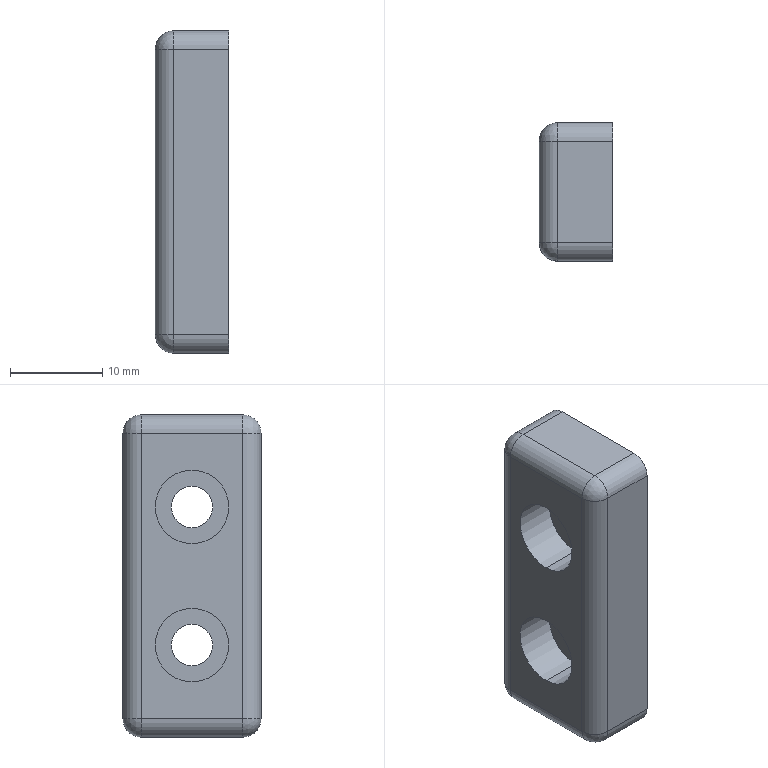Part | STEP file | 0246_219_Block | 1 solid | 28 faces | box 8 x 15 x 35 mm | volume 3528 mm3 | cylinder 16 | plane 8 | sphere 4 | commonest cylinder face diameters 4 x8 4.5 x4 8 x4